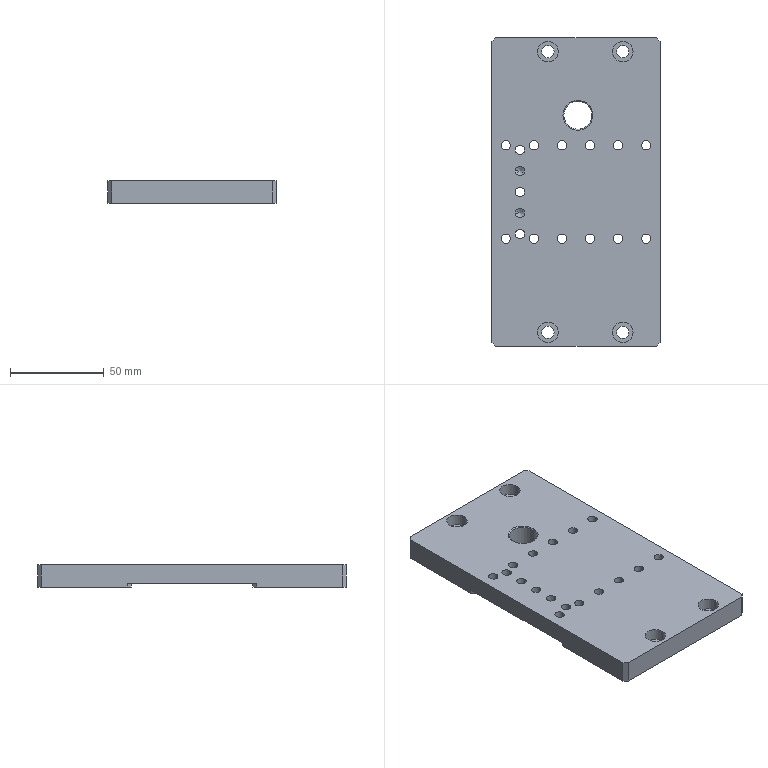Part | 1 solid | 90 faces | box 90 x 165 x 12 mm | volume 157233 mm3 | cylinder 56 | plane 22 | cone 12 | commonest cylinder face diameters 5 x38 6.6 x8 11 x8 15 x2